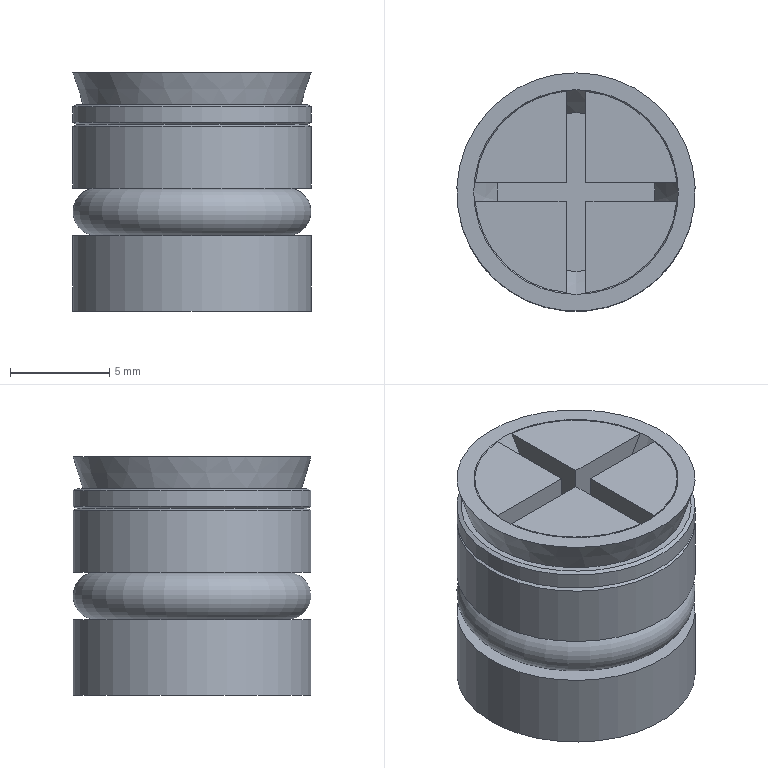Part | STEP file | EC31200008 | 1 solid | 31 faces | box 12 x 12 x 12 mm | volume 1282 mm3 | plane 14 | cone 9 | spline 4 | cylinder 3 | torus 1 | commonest cylinder face diameters 12 x3